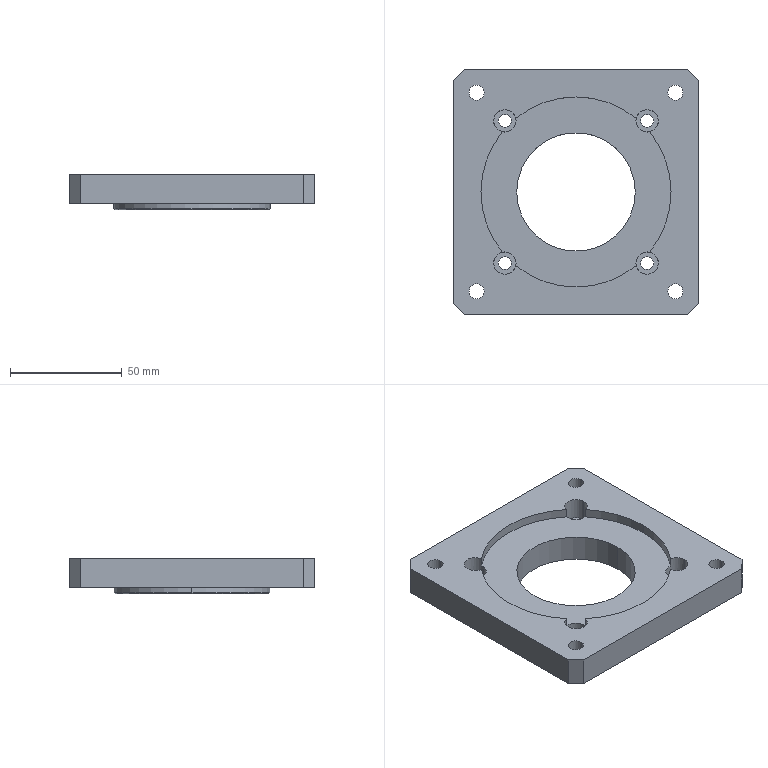Part | SolidWorks | features ICE 3, Chamfer 2, HoleWzd 2, Extrusion 1 | 1 solid | 51 faces | box 110 x 110 x 16 mm | volume 113885 mm3 | cylinder 33 | plane 16 | cone 2 | commonest cylinder face diameters 5.8 x8 6.8 x8 10 x8 85 x5 53 x2 70 x2